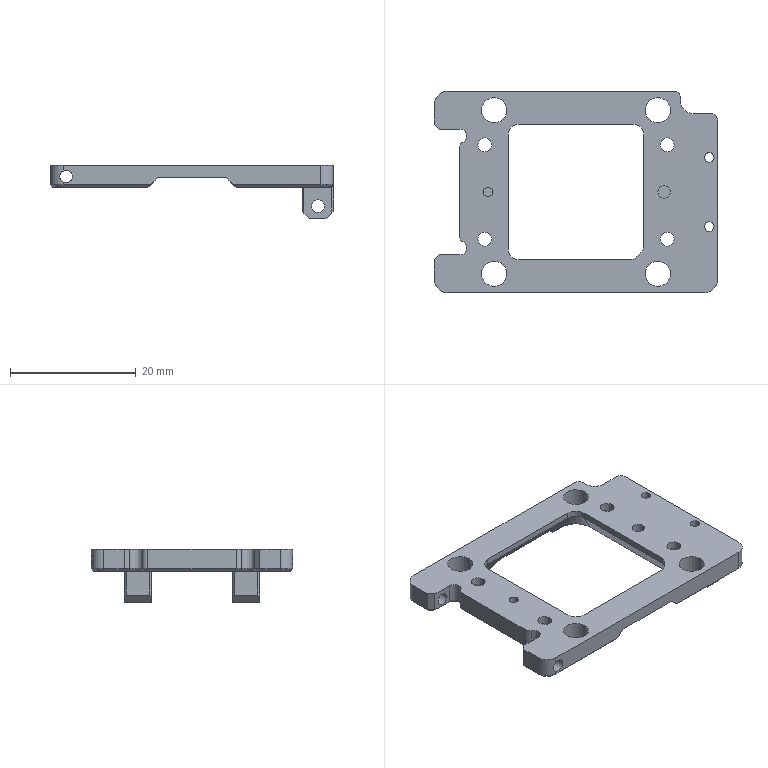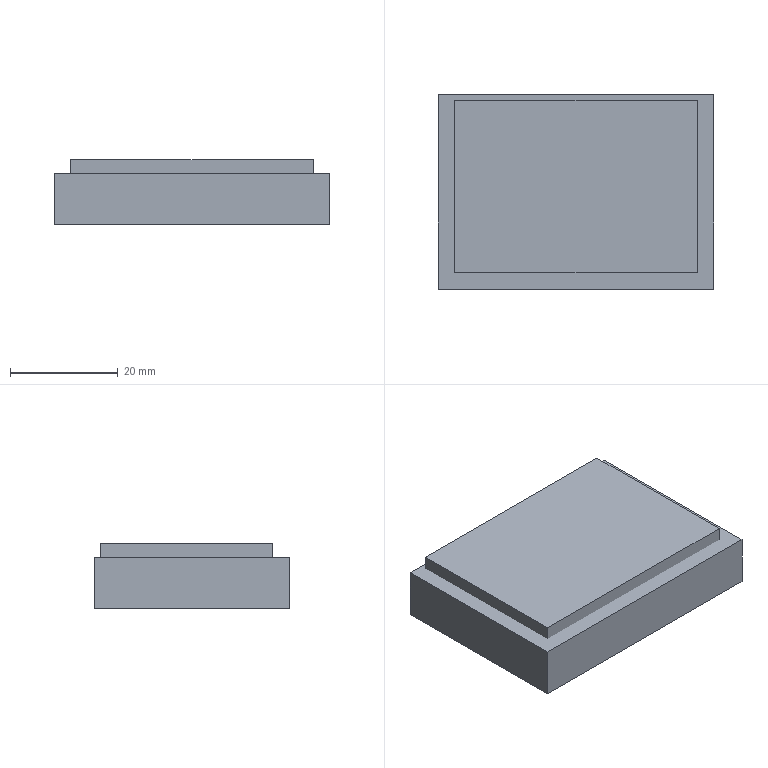CAM job | NX | 3+2 milling, drilling | part box 45 x 32 x 8.5 mm | stock box 51 x 36 x 12 mm
Tools:
number,name,description,diameter,corner_radius,flute_length,length,flutes
3,D63,Milling Tool-5 Parameters,63.0,0.0,50.0,75.0,2
1,D6A45,Milling Tool-5 Parameters,6.0,0.0,50.0,75.0,2
9,4.0ZT,Drilling Tool,4.0,0.0,35.0,50.0,2
12,2.2ZT,Drilling Tool,2.2,0.0,35.0,50.0,2
20,1.5ZT,Drilling Tool,1.5,0.0,35.0,50.0,2
6,D6,Milling Tool-5 Parameters,6.0,0.0,50.0,75.0,2
17,D3,Milling Tool-5 Parameters,3.0,0.0,50.0,75.0,2
19,D1.5,Milling Tool-5 Parameters,1.5,0.0,50.0,75.0,2
21,D1,Milling Tool-5 Parameters,1.0,0.0,50.0,75.0,2
16,D6JING,Milling Tool-5 Parameters,6.0,0.0,50.0,75.0,2
7,D3R0.5,Milling Tool-5 Parameters,3.0,0.5,50.0,75.0,2
15,R0.75,Milling Tool-5 Parameters,0.05,0.025,50.0,75.0,2
18,2.02ZT,Drilling Tool,2.02,0.0,35.0,50.0,2
14,D4A45,Milling Tool-5 Parameters,4.0,0.0,50.0,75.0,2
Operations:
program,operation,operation_type,tool,method,geometry_group,spindle_rpm,surface_speed,feed_per_tooth,feed_cut,feed_plunge,cut_length_mm,path_length_mm,cut_time_min,machine_time_min
1,FLOOR_WALL,VolumeBased25DMillingOperation,D63,METHOD,A,6500.0,1286.0,0.0962,1250.0,100.0,126.0,180.0,0.1008,0.1062
1,DRILLING,Operation,D6A45,METHOD,A,5000.0,94.0,0.025,250.0,0.0,43.2,281.832,0.1728,0.1967
1,DRILLING_COPY_COPY,Operation,2.2ZT,METHOD,A,1447.0,10.0,0.0346,100.0,0.0,25.844,180.436,0.2584,0.2739
1,DRILLING_COPY_COPY_1,Operation,1.5ZT,METHOD,A,2000.0,10.0,0.025,100.0,0.0,16.901,108.204,0.169,0.1781
1,DRILLING_COPY_COPY_COPY,Operation,4.0ZT,METHOD,A,1447.0,10.0,0.0346,100.0,0.0,36.807,221.131,0.3681,0.3865
1,ADAPTIVE_MILLING,CavityMilling,D6,METHOD,A,9500.0,179.0,0.1579,3000.0,1000.0,2824.623,2987.731,1.396,1.412
1,CAVITY_MILL,CavityMilling,D3,METHOD,A,9500.0,89.0,0.0579,1100.0,100.0,1506.722,3433.104,1.37,1.562
1,ZLEVEL_PROFILE,ZLevelMilling,D3,METHOD,A,9500.0,89.0,0.0526,1000.0,100.0,341.308,415.429,0.3413,0.3487
1,ZLEVEL_PROFILE_COPY,ZLevelMilling,D3,METHOD,A,9500.0,89.0,0.0526,1000.0,100.0,78.387,137.387,0.0784,0.0843
1,CAVITY_MILL_COPY,CavityMilling,D1.5,METHOD,A,9500.0,44.0,0.05,950.0,100.0,223.307,448.599,0.2351,0.2576
1,HOLE_MILLING_COPY_COPY,CylinderMilling,D1,METHOD,A,9506.0,29.0,0.0342,650.0,100.0,154.522,306.522,0.2377,0.2529
1,PLANAR_MILL,PlanarMilling,D6A45,METHOD,A,9500.0,179.0,0.0658,1250.0,100.0,326.986,1088.842,0.2616,0.3378
1,CUTTERCOMP21.,CylinderMilling,D1,METHOD,A,9506.0,29.0,0.0342,650.0,100.0,90.672,242.672,0.1395,0.1547
2,FLOOR_WALL_COPY,VolumeBased25DMillingOperation,D63,METHOD,B,6500.0,1286.0,0.0962,1250.0,100.0,480.0,1027.501,0.384,0.4388
2,FLOOR_WALL_2,VolumeBased25DMillingOperation,D6,METHOD,B,9500.0,179.0,0.1316,2500.0,1000.0,6894.045,7135.72,2.779,2.803
2,FLOOR_WALL_2_COPY,VolumeBased25DMillingOperation,D6,METHOD,B,9500.0,179.0,0.1316,2500.0,1000.0,231.953,426.496,0.1061,0.1256
2,FLOOR_WALL_1_COPY_COPY,VolumeBased25DMillingOperation,D6JING,METHOD,B,9500.0,89.0,0.0526,1000.0,100.0,682.991,1597.245,0.683,0.7744
2,HOLE_MILLING,CylinderMilling,D3,METHOD,B,9500.0,89.0,0.0658,1250.0,100.0,188.839,534.639,0.1511,0.1857
2,PLANAR_MILL_COPY,PlanarMilling,D6A45,METHOD,B,9500.0,179.0,0.0658,1250.0,100.0,62.721,203.571,0.0502,0.0643
2,PLANAR_MILL_COPY_COPY,PlanarMilling,D6A45,METHOD,B,9500.0,179.0,0.0658,1250.0,100.0,150.63,299.87,0.1205,0.1354
2,PLANAR_MILL_COPY_COPY_COPY,PlanarMilling,D6A45,METHOD,B,9500.0,179.0,0.0658,1250.0,100.0,91.669,729.921,0.0733,0.1372
2,ZLEVEL_PROFILE_1,ZLevelMilling,D3R0.5,METHOD,B,9500.0,89.0,0.1316,2500.0,1000.0,2424.458,2799.474,0.9767,1.014
2,ZLEVEL_PROFILE_1_COPY,ZLevelMilling,D3R0.5,METHOD,B,9500.0,89.0,0.1316,2500.0,1000.0,471.439,793.846,0.1941,0.2263
2,ZLEVEL_PROFILE_2_COPY,ZLevelMilling,R0.75,METHOD,MCS_MILL_COPY,9500.0,14.0,0.0658,1250.0,500.0,32.345,226.548,0.0371,0.0565
3,DRILLING_COPY,Operation,D4A45,METHOD,C,5000.0,94.0,0.025,250.0,0.0,8.2,124.988,0.0328,0.0445
3,DRILLING_COPY_COPY_COPY_1,Operation,2.02ZT,METHOD,C,1447.0,10.0,0.0346,100.0,0.0,20.464,149.516,0.2046,0.2175
4,DRILLING_COPY_COPY_2,Operation,D4A45,METHOD,D,5000.0,94.0,0.025,250.0,0.0,8.2,124.988,0.0328,0.0445
4,DRILLING_COPY_COPY_COPY_1_COPY,Operation,2.02ZT,METHOD,D,1447.0,10.0,0.0346,100.0,0.0,20.464,150.289,0.2046,0.2176